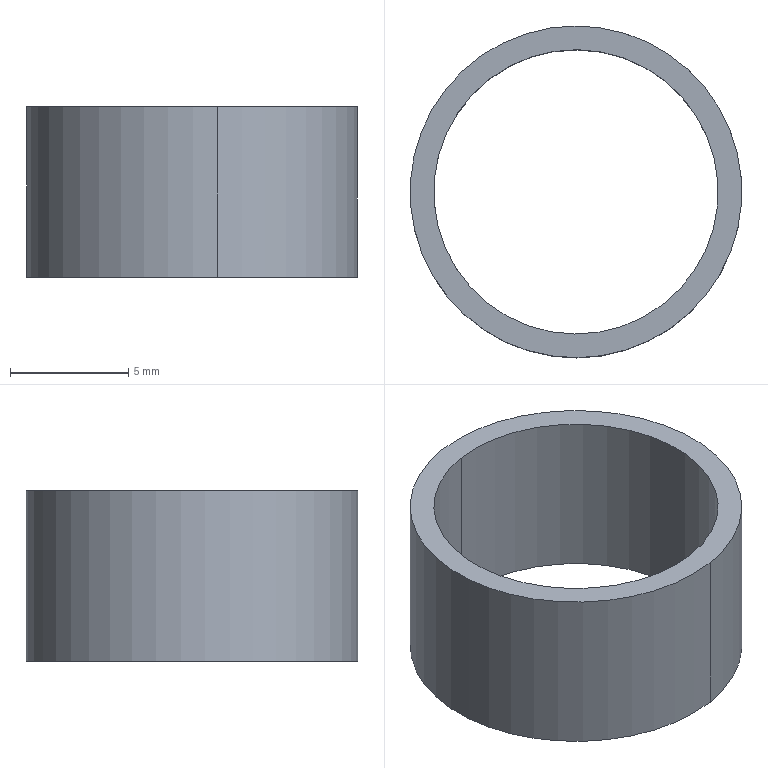Part | SolidWorks | features BaseBody 1 | 1 solid | 6 faces | box 14.001 x 14 x 7.202 mm | volume 294.053 mm3 | cylinder 4 | plane 2 | commonest cylinder face diameters 12 x2 14 x2
STEP:
#1=CARTESIAN_POINT('',(342.698,191.476,14.275));
#2=VERTEX_POINT('',#1);
#3=CARTESIAN_POINT('',(340.841,203.331,14.274));
#4=VERTEX_POINT('',#3);
#5=CARTESIAN_POINT('',(341.77,197.404,14.275));
#6=DIRECTION('',(0.0001435,0.000000521,-1.));
#7=DIRECTION('',(-1.,0.,-0.0001435));
#8=AXIS2_PLACEMENT_3D('',#5,#6,#7);
#9=CIRCLE('',#8,6.);
#10=EDGE_CURVE('',#2,#4,#9,.T.);
#11=ORIENTED_EDGE('',*,*,#10,.F.);
#12=CARTESIAN_POINT('',(342.699,191.476,7.075));
#13=VERTEX_POINT('',#12);
#14=CARTESIAN_POINT('',(342.698,191.476,14.275));
#15=DIRECTION('',(0.0001435,0.000000521,-1.));
#16=VECTOR('',#15,1000.);
#17=LINE('',#14,#16);
#18=EDGE_CURVE('',#2,#13,#17,.T.);
#19=ORIENTED_EDGE('',*,*,#18,.T.);
#20=CARTESIAN_POINT('',(340.842,203.331,7.074));
#21=VERTEX_POINT('',#20);
#22=CARTESIAN_POINT('',(341.771,197.404,7.075));
#23=DIRECTION('',(-0.0001435,-0.000000521,1.));
#24=DIRECTION('',(0.1548,-0.988,0.00002169));
#25=AXIS2_PLACEMENT_3D('',#22,#23,#24);
#26=CIRCLE('',#25,6.);
#27=EDGE_CURVE('',#21,#13,#26,.T.);
#28=ORIENTED_EDGE('',*,*,#27,.F.);
#29=CARTESIAN_POINT('',(340.841,203.331,14.274));
#30=DIRECTION('',(0.0001435,0.000000521,-1.));
#31=VECTOR('',#30,1000.);
#32=LINE('',#29,#31);
#33=EDGE_CURVE('',#4,#21,#32,.T.);
#34=ORIENTED_EDGE('',*,*,#33,.F.);
#35=EDGE_LOOP('',(#11,#19,#28,#34));
#36=FACE_OUTER_BOUND('',#35,.T.);
#37=CARTESIAN_POINT('',(341.77,197.404,14.275));
#38=DIRECTION('',(0.0001435,0.000000521,-1.));
#39=DIRECTION('',(-0.1548,0.988,-0.00002169));
#40=AXIS2_PLACEMENT_3D('',#37,#38,#39);
#41=CYLINDRICAL_SURFACE('',#40,6.);
#42=ADVANCED_FACE('',(#36),#41,.F.);
#43=CARTESIAN_POINT('',(342.853,190.488,14.275));
#44=VERTEX_POINT('',#43);
#45=CARTESIAN_POINT('',(340.686,204.319,14.274));
#46=VERTEX_POINT('',#45);
#47=CARTESIAN_POINT('',(341.77,197.404,14.275));
#48=DIRECTION('',(-0.0001435,-0.000000521,1.));
#49=DIRECTION('',(0.1548,-0.988,0.00002169));
#50=AXIS2_PLACEMENT_3D('',#47,#48,#49);
#51=CIRCLE('',#50,7.);
#52=EDGE_CURVE('',#44,#46,#51,.T.);
#53=ORIENTED_EDGE('',*,*,#52,.F.);
#54=CARTESIAN_POINT('',(342.854,190.488,7.075));
#55=VERTEX_POINT('',#54);
#56=CARTESIAN_POINT('',(342.853,190.488,14.275));
#57=DIRECTION('',(0.0001435,0.000000521,-1.));
#58=VECTOR('',#57,1000.);
#59=LINE('',#56,#58);
#60=EDGE_CURVE('',#44,#55,#59,.T.);
#61=ORIENTED_EDGE('',*,*,#60,.T.);
#62=CARTESIAN_POINT('',(340.687,204.319,7.074));
#63=VERTEX_POINT('',#62);
#64=CARTESIAN_POINT('',(341.771,197.404,7.075));
#65=DIRECTION('',(0.0001435,0.000000521,-1.));
#66=DIRECTION('',(0.1548,-0.988,0.00002169));
#67=AXIS2_PLACEMENT_3D('',#64,#65,#66);
#68=CIRCLE('',#67,7.);
#69=EDGE_CURVE('',#63,#55,#68,.T.);
#70=ORIENTED_EDGE('',*,*,#69,.F.);
#71=CARTESIAN_POINT('',(340.686,204.319,14.274));
#72=DIRECTION('',(0.0001435,0.000000521,-1.));
#73=VECTOR('',#72,1000.);
#74=LINE('',#71,#73);
#75=EDGE_CURVE('',#46,#63,#74,.T.);
#76=ORIENTED_EDGE('',*,*,#75,.F.);
#77=EDGE_LOOP('',(#53,#61,#70,#76));
#78=FACE_OUTER_BOUND('',#77,.T.);
#79=CARTESIAN_POINT('',(341.77,197.404,14.275));
#80=DIRECTION('',(0.0001435,0.000000521,-1.));
#81=DIRECTION('',(-0.1548,0.988,-0.00002169));
#82=AXIS2_PLACEMENT_3D('',#79,#80,#81);
#83=CYLINDRICAL_SURFACE('',#82,7.);
#84=ADVANCED_FACE('',(#78),#83,.T.);
#85=ORIENTED_EDGE('',*,*,#60,.F.);
#86=CARTESIAN_POINT('',(341.77,197.404,14.275));
#87=DIRECTION('',(-0.0001435,-0.000000521,1.));
#88=DIRECTION('',(0.1548,-0.988,0.00002169));
#89=AXIS2_PLACEMENT_3D('',#86,#87,#88);
#90=CIRCLE('',#89,7.);
#91=EDGE_CURVE('',#46,#44,#90,.T.);
#92=ORIENTED_EDGE('',*,*,#91,.F.);
#93=ORIENTED_EDGE('',*,*,#75,.T.);
#94=CARTESIAN_POINT('',(341.771,197.404,7.075));
#95=DIRECTION('',(0.0001435,0.000000521,-1.));
#96=DIRECTION('',(0.1548,-0.988,0.00002169));
#97=AXIS2_PLACEMENT_3D('',#94,#95,#96);
#98=CIRCLE('',#97,7.);
#99=EDGE_CURVE('',#55,#63,#98,.T.);
#100=ORIENTED_EDGE('',*,*,#99,.F.);
#101=EDGE_LOOP('',(#85,#92,#93,#100));
#102=FACE_OUTER_BOUND('',#101,.T.);
#103=CARTESIAN_POINT('',(341.77,197.404,14.275));
#104=DIRECTION('',(0.0001435,0.000000521,-1.));
#105=DIRECTION('',(-0.1548,0.988,-0.00002169));
#106=AXIS2_PLACEMENT_3D('',#103,#104,#105);
#107=CYLINDRICAL_SURFACE('',#106,7.);
#108=ADVANCED_FACE('',(#102),#107,.T.);
#109=CARTESIAN_POINT('',(341.77,197.404,14.275));
#110=DIRECTION('',(0.0001435,0.000000521,-1.));
#111=DIRECTION('',(-1.,0.,-0.0001435));
#112=AXIS2_PLACEMENT_3D('',#109,#110,#111);
#113=CIRCLE('',#112,6.);
#114=EDGE_CURVE('',#4,#2,#113,.T.);
#115=ORIENTED_EDGE('',*,*,#114,.T.);
#116=ORIENTED_EDGE('',*,*,#10,.T.);
#117=EDGE_LOOP('',(#115,#116));
#118=FACE_BOUND('',#117,.T.);
#119=ORIENTED_EDGE('',*,*,#91,.T.);
#120=ORIENTED_EDGE('',*,*,#52,.T.);
#121=EDGE_LOOP('',(#119,#120));
#122=FACE_OUTER_BOUND('',#121,.T.);
#123=CARTESIAN_POINT('',(341.77,197.404,14.275));
#124=DIRECTION('',(-0.0001435,-0.000000521,1.));
#125=DIRECTION('',(-0.003633,1.,0.));
#126=AXIS2_PLACEMENT_3D('',#123,#124,#125);
#127=PLANE('',#126);
#128=ADVANCED_FACE('',(#118,#122),#127,.T.);
#129=ORIENTED_EDGE('',*,*,#18,.F.);
#130=ORIENTED_EDGE('',*,*,#114,.F.);
#131=ORIENTED_EDGE('',*,*,#33,.T.);
#132=CARTESIAN_POINT('',(341.771,197.404,7.075));
#133=DIRECTION('',(-0.0001435,-0.000000521,1.));
#134=DIRECTION('',(0.1548,-0.988,0.00002169));
#135=AXIS2_PLACEMENT_3D('',#132,#133,#134);
#136=CIRCLE('',#135,6.);
#137=EDGE_CURVE('',#13,#21,#136,.T.);
#138=ORIENTED_EDGE('',*,*,#137,.F.);
#139=EDGE_LOOP('',(#129,#130,#131,#138));
#140=FACE_OUTER_BOUND('',#139,.T.);
#141=CARTESIAN_POINT('',(341.77,197.404,14.275));
#142=DIRECTION('',(0.0001435,0.000000521,-1.));
#143=DIRECTION('',(-0.1548,0.988,-0.00002169));
#144=AXIS2_PLACEMENT_3D('',#141,#142,#143);
#145=CYLINDRICAL_SURFACE('',#144,6.);
#146=ADVANCED_FACE('',(#140),#145,.F.);
#147=ORIENTED_EDGE('',*,*,#27,.T.);
#148=ORIENTED_EDGE('',*,*,#137,.T.);
#149=EDGE_LOOP('',(#147,#148));
#150=FACE_BOUND('',#149,.T.);
#151=ORIENTED_EDGE('',*,*,#69,.T.);
#152=ORIENTED_EDGE('',*,*,#99,.T.);
#153=EDGE_LOOP('',(#151,#152));
#154=FACE_OUTER_BOUND('',#153,.T.);
#155=CARTESIAN_POINT('',(341.771,197.404,7.075));
#156=DIRECTION('',(0.0001435,0.000000521,-1.));
#157=DIRECTION('',(0.,-1.,-0.000000521));
#158=AXIS2_PLACEMENT_3D('',#155,#156,#157);
#159=PLANE('',#158);
#160=ADVANCED_FACE('',(#150,#154),#159,.T.);
#161=CLOSED_SHELL('',(#42,#84,#108,#128,#146,#160));
#162=MANIFOLD_SOLID_BREP('',#161);
#163=CARTESIAN_POINT('',(0.,0.,0.));
#164=DIRECTION('',(0.,0.,1.));
#165=DIRECTION('',(1.,0.,0.));
#166=AXIS2_PLACEMENT_3D('',#163,#164,#165);
#167=(LENGTH_UNIT()NAMED_UNIT(*)SI_UNIT(.MILLI.,.METRE.));
#168=UNCERTAINTY_MEASURE_WITH_UNIT(LENGTH_MEASURE(0.00001),#167,'','');
#169=(NAMED_UNIT(*)PLANE_ANGLE_UNIT()SI_UNIT($,.RADIAN.));
#170=(NAMED_UNIT(*)SI_UNIT($,.STERADIAN.)SOLID_ANGLE_UNIT());
#171=(GEOMETRIC_REPRESENTATION_CONTEXT(3)GLOBAL_UNCERTAINTY_ASSIGNED_CONTEXT((#168))GLOBAL_UNIT_ASSIGNED_CONTEXT((#167,#169,#170))REPRESENTATION_CONTEXT('',''));
#172=ADVANCED_BREP_SHAPE_REPRESENTATION('',(#162,#166),#171);